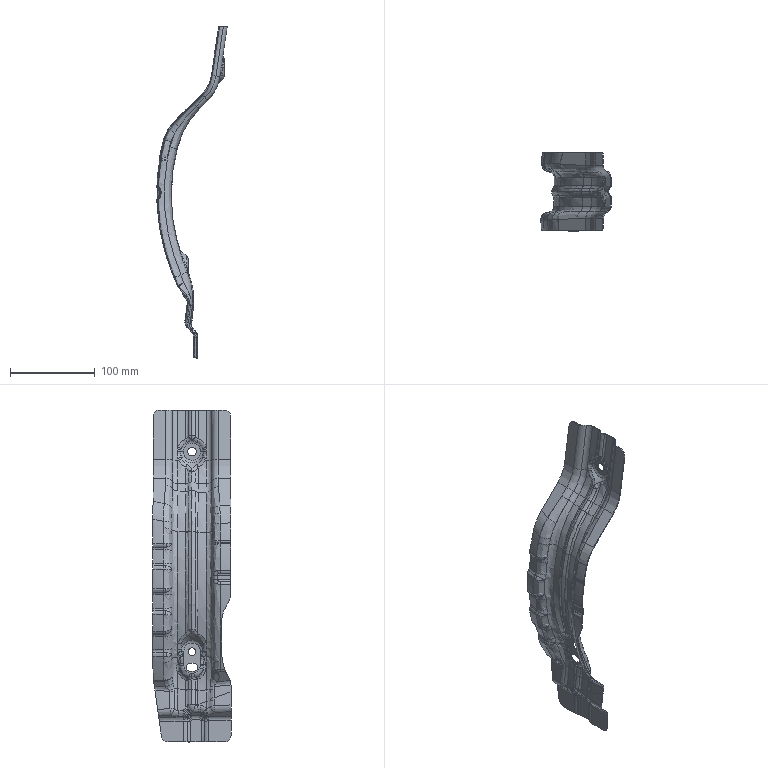Part | 1 solid | 817 faces | box 83.134 x 92.399 x 392.145 mm | volume 42327 mm3 | spline 633 | cylinder 100 | plane 44 | sphere 24 | torus 16 | commonest cylinder face diameters 16 x25 10 x14 18 x13 14 x12 8 x10 9 x4